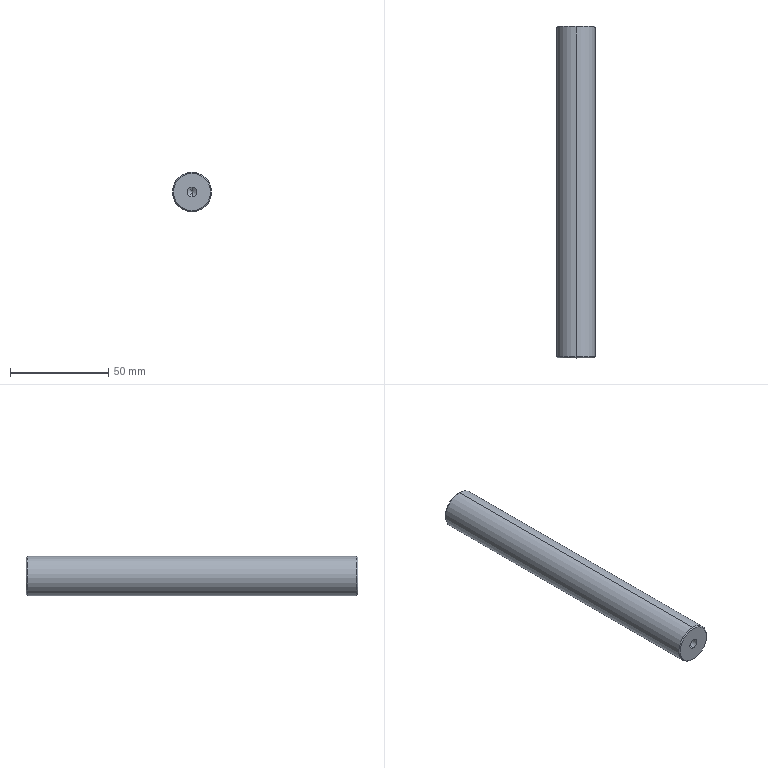Part | SolidWorks | features BaseBody 1 | 1 solid | 16 faces | box 20 x 169 x 20 mm | volume 51704 mm3 | cone 8 | cylinder 6 | plane 2 | commonest cylinder face diameters 5 x2 6.8 x2 20 x2
STEP:
#1=CARTESIAN_POINT('',(0.,15.,2.5));
#2=VERTEX_POINT('',#1);
#3=CARTESIAN_POINT('',(0.,15.,-2.5));
#4=VERTEX_POINT('',#3);
#5=CARTESIAN_POINT('',(0.,15.,0.));
#6=DIRECTION('',(0.,-1.,0.));
#7=DIRECTION('',(0.,0.,-1.));
#8=AXIS2_PLACEMENT_3D('',#5,#6,#7);
#9=CIRCLE('',#8,2.5);
#10=EDGE_CURVE('',#2,#4,#9,.T.);
#11=ORIENTED_EDGE('',*,*,#10,.F.);
#12=CARTESIAN_POINT('',(0.,0.,2.5));
#13=VERTEX_POINT('',#12);
#14=CARTESIAN_POINT('',(0.,0.,2.5));
#15=DIRECTION('',(0.,-1.,0.));
#16=VECTOR('',#15,1000.);
#17=LINE('',#14,#16);
#18=EDGE_CURVE('',#2,#13,#17,.T.);
#19=ORIENTED_EDGE('',*,*,#18,.T.);
#20=CARTESIAN_POINT('',(0.,0.,-2.5));
#21=VERTEX_POINT('',#20);
#22=CARTESIAN_POINT('',(0.,0.,0.));
#23=DIRECTION('',(0.,-1.,0.));
#24=DIRECTION('',(0.,0.,-1.));
#25=AXIS2_PLACEMENT_3D('',#22,#23,#24);
#26=CIRCLE('',#25,2.5);
#27=EDGE_CURVE('',#13,#21,#26,.T.);
#28=ORIENTED_EDGE('',*,*,#27,.T.);
#29=CARTESIAN_POINT('',(0.,0.,-2.5));
#30=DIRECTION('',(0.,-1.,0.));
#31=VECTOR('',#30,1000.);
#32=LINE('',#29,#31);
#33=EDGE_CURVE('',#4,#21,#32,.T.);
#34=ORIENTED_EDGE('',*,*,#33,.F.);
#35=EDGE_LOOP('',(#11,#19,#28,#34));
#36=FACE_OUTER_BOUND('',#35,.T.);
#37=CARTESIAN_POINT('',(0.,0.,0.));
#38=DIRECTION('',(0.,-1.,0.));
#39=DIRECTION('',(0.,0.,-1.));
#40=AXIS2_PLACEMENT_3D('',#37,#38,#39);
#41=CYLINDRICAL_SURFACE('',#40,2.5);
#42=ADVANCED_FACE('',(#36),#41,.F.);
#43=CARTESIAN_POINT('',(0.,16.502,0.));
#44=VERTEX_POINT('',#43);
#45=CARTESIAN_POINT('',(0.,15.,-2.5));
#46=DIRECTION('',(0.,-0.515,-0.8572));
#47=VECTOR('',#46,1000.);
#48=LINE('',#45,#47);
#49=EDGE_CURVE('',#44,#4,#48,.T.);
#50=ORIENTED_EDGE('',*,*,#49,.F.);
#51=CARTESIAN_POINT('',(0.,15.,2.5));
#52=DIRECTION('',(0.,-0.515,0.8572));
#53=VECTOR('',#52,1000.);
#54=LINE('',#51,#53);
#55=EDGE_CURVE('',#44,#2,#54,.T.);
#56=ORIENTED_EDGE('',*,*,#55,.T.);
#57=ORIENTED_EDGE('',*,*,#10,.T.);
#58=EDGE_LOOP('',(#50,#56,#57));
#59=FACE_OUTER_BOUND('',#58,.T.);
#60=CARTESIAN_POINT('',(0.,15.,0.));
#61=DIRECTION('',(0.,-1.,0.));
#62=DIRECTION('',(0.,0.,-1.));
#63=AXIS2_PLACEMENT_3D('',#60,#61,#62);
#64=CONICAL_SURFACE('',#63,2.5,1.03);
#65=ADVANCED_FACE('',(#59),#64,.F.);
#66=CARTESIAN_POINT('',(0.,140.25,-3.4));
#67=VERTEX_POINT('',#66);
#68=CARTESIAN_POINT('',(0.,140.25,3.4));
#69=VERTEX_POINT('',#68);
#70=CARTESIAN_POINT('',(0.,140.25,0.));
#71=DIRECTION('',(0.,1.,0.));
#72=DIRECTION('',(0.,0.,1.));
#73=AXIS2_PLACEMENT_3D('',#70,#71,#72);
#74=CIRCLE('',#73,3.4);
#75=EDGE_CURVE('',#67,#69,#74,.T.);
#76=ORIENTED_EDGE('',*,*,#75,.F.);
#77=CARTESIAN_POINT('',(0.,169.,-3.4));
#78=VERTEX_POINT('',#77);
#79=CARTESIAN_POINT('',(0.,169.,-3.4));
#80=DIRECTION('',(0.,1.,0.));
#81=VECTOR('',#80,1000.);
#82=LINE('',#79,#81);
#83=EDGE_CURVE('',#67,#78,#82,.T.);
#84=ORIENTED_EDGE('',*,*,#83,.T.);
#85=CARTESIAN_POINT('',(0.,169.,3.4));
#86=VERTEX_POINT('',#85);
#87=CARTESIAN_POINT('',(0.,169.,0.));
#88=DIRECTION('',(0.,1.,0.));
#89=DIRECTION('',(0.,0.,1.));
#90=AXIS2_PLACEMENT_3D('',#87,#88,#89);
#91=CIRCLE('',#90,3.4);
#92=EDGE_CURVE('',#78,#86,#91,.T.);
#93=ORIENTED_EDGE('',*,*,#92,.T.);
#94=CARTESIAN_POINT('',(0.,169.,3.4));
#95=DIRECTION('',(0.,1.,0.));
#96=VECTOR('',#95,1000.);
#97=LINE('',#94,#96);
#98=EDGE_CURVE('',#69,#86,#97,.T.);
#99=ORIENTED_EDGE('',*,*,#98,.F.);
#100=EDGE_LOOP('',(#76,#84,#93,#99));
#101=FACE_OUTER_BOUND('',#100,.T.);
#102=CARTESIAN_POINT('',(0.,169.,0.));
#103=DIRECTION('',(0.,1.,0.));
#104=DIRECTION('',(0.,0.,1.));
#105=AXIS2_PLACEMENT_3D('',#102,#103,#104);
#106=CYLINDRICAL_SURFACE('',#105,3.4);
#107=ADVANCED_FACE('',(#101),#106,.F.);
#108=CARTESIAN_POINT('',(0.,138.207,0.));
#109=VERTEX_POINT('',#108);
#110=CARTESIAN_POINT('',(0.,140.25,3.4));
#111=DIRECTION('',(0.,0.515,0.8572));
#112=VECTOR('',#111,1000.);
#113=LINE('',#110,#112);
#114=EDGE_CURVE('',#109,#69,#113,.T.);
#115=ORIENTED_EDGE('',*,*,#114,.F.);
#116=CARTESIAN_POINT('',(0.,140.25,-3.4));
#117=DIRECTION('',(0.,0.515,-0.8572));
#118=VECTOR('',#117,1000.);
#119=LINE('',#116,#118);
#120=EDGE_CURVE('',#109,#67,#119,.T.);
#121=ORIENTED_EDGE('',*,*,#120,.T.);
#122=ORIENTED_EDGE('',*,*,#75,.T.);
#123=EDGE_LOOP('',(#115,#121,#122));
#124=FACE_OUTER_BOUND('',#123,.T.);
#125=CARTESIAN_POINT('',(0.,140.25,0.));
#126=DIRECTION('',(0.,1.,0.));
#127=DIRECTION('',(0.,0.,1.));
#128=AXIS2_PLACEMENT_3D('',#125,#126,#127);
#129=CONICAL_SURFACE('',#128,3.4,1.03);
#130=ADVANCED_FACE('',(#124),#129,.F.);
#131=CARTESIAN_POINT('',(0.,169.,9.5));
#132=VERTEX_POINT('',#131);
#133=CARTESIAN_POINT('',(0.,169.,-9.5));
#134=VERTEX_POINT('',#133);
#135=CARTESIAN_POINT('',(0.,169.,0.));
#136=DIRECTION('',(0.,1.,0.));
#137=DIRECTION('',(0.,0.,1.));
#138=AXIS2_PLACEMENT_3D('',#135,#136,#137);
#139=CIRCLE('',#138,9.5);
#140=EDGE_CURVE('',#132,#134,#139,.T.);
#141=ORIENTED_EDGE('',*,*,#140,.F.);
#142=CARTESIAN_POINT('',(0.,168.5,10.));
#143=VERTEX_POINT('',#142);
#144=CARTESIAN_POINT('',(0.,169.,9.5));
#145=DIRECTION('',(0.,-0.7071,0.7071));
#146=VECTOR('',#145,1000.);
#147=LINE('',#144,#146);
#148=EDGE_CURVE('',#132,#143,#147,.T.);
#149=ORIENTED_EDGE('',*,*,#148,.T.);
#150=CARTESIAN_POINT('',(0.,168.5,-10.));
#151=VERTEX_POINT('',#150);
#152=CARTESIAN_POINT('',(0.,168.5,0.));
#153=DIRECTION('',(0.,-1.,0.));
#154=DIRECTION('',(0.,0.,1.));
#155=AXIS2_PLACEMENT_3D('',#152,#153,#154);
#156=CIRCLE('',#155,10.);
#157=EDGE_CURVE('',#151,#143,#156,.T.);
#158=ORIENTED_EDGE('',*,*,#157,.F.);
#159=CARTESIAN_POINT('',(0.,169.,-9.5));
#160=DIRECTION('',(0.,-0.7071,-0.7071));
#161=VECTOR('',#160,1000.);
#162=LINE('',#159,#161);
#163=EDGE_CURVE('',#134,#151,#162,.T.);
#164=ORIENTED_EDGE('',*,*,#163,.F.);
#165=EDGE_LOOP('',(#141,#149,#158,#164));
#166=FACE_OUTER_BOUND('',#165,.T.);
#167=CARTESIAN_POINT('',(0.,169.,0.));
#168=DIRECTION('',(0.,-1.,0.));
#169=DIRECTION('',(0.,0.,-1.));
#170=AXIS2_PLACEMENT_3D('',#167,#168,#169);
#171=CONICAL_SURFACE('',#170,9.5,0.7854);
#172=ADVANCED_FACE('',(#166),#171,.T.);
#173=CARTESIAN_POINT('',(0.,0.,-9.5));
#174=VERTEX_POINT('',#173);
#175=CARTESIAN_POINT('',(0.,0.,9.5));
#176=VERTEX_POINT('',#175);
#177=CARTESIAN_POINT('',(0.,0.,0.));
#178=DIRECTION('',(0.,-1.,0.));
#179=DIRECTION('',(0.,0.,1.));
#180=AXIS2_PLACEMENT_3D('',#177,#178,#179);
#181=CIRCLE('',#180,9.5);
#182=EDGE_CURVE('',#174,#176,#181,.T.);
#183=ORIENTED_EDGE('',*,*,#182,.F.);
#184=CARTESIAN_POINT('',(0.,0.5,-10.));
#185=VERTEX_POINT('',#184);
#186=CARTESIAN_POINT('',(0.,0.5,-10.));
#187=DIRECTION('',(0.,0.7071,-0.7071));
#188=VECTOR('',#187,1000.);
#189=LINE('',#186,#188);
#190=EDGE_CURVE('',#174,#185,#189,.T.);
#191=ORIENTED_EDGE('',*,*,#190,.T.);
#192=CARTESIAN_POINT('',(0.,0.5,10.));
#193=VERTEX_POINT('',#192);
#194=CARTESIAN_POINT('',(0.,0.5,0.));
#195=DIRECTION('',(0.,1.,0.));
#196=DIRECTION('',(0.,0.,1.));
#197=AXIS2_PLACEMENT_3D('',#194,#195,#196);
#198=CIRCLE('',#197,10.);
#199=EDGE_CURVE('',#193,#185,#198,.T.);
#200=ORIENTED_EDGE('',*,*,#199,.F.);
#201=CARTESIAN_POINT('',(0.,0.5,10.));
#202=DIRECTION('',(0.,0.7071,0.7071));
#203=VECTOR('',#202,1000.);
#204=LINE('',#201,#203);
#205=EDGE_CURVE('',#176,#193,#204,.T.);
#206=ORIENTED_EDGE('',*,*,#205,.F.);
#207=EDGE_LOOP('',(#183,#191,#200,#206));
#208=FACE_OUTER_BOUND('',#207,.T.);
#209=CARTESIAN_POINT('',(0.,0.5,0.));
#210=DIRECTION('',(0.,1.,0.));
#211=DIRECTION('',(0.,0.,1.));
#212=AXIS2_PLACEMENT_3D('',#209,#210,#211);
#213=CONICAL_SURFACE('',#212,10.,0.7854);
#214=ADVANCED_FACE('',(#208),#213,.T.);
#215=ORIENTED_EDGE('',*,*,#157,.T.);
#216=CARTESIAN_POINT('',(0.,169.,10.));
#217=DIRECTION('',(0.,-1.,0.));
#218=VECTOR('',#217,1000.);
#219=LINE('',#216,#218);
#220=EDGE_CURVE('',#143,#193,#219,.T.);
#221=ORIENTED_EDGE('',*,*,#220,.T.);
#222=ORIENTED_EDGE('',*,*,#199,.T.);
#223=CARTESIAN_POINT('',(0.,169.,-10.));
#224=DIRECTION('',(0.,-1.,0.));
#225=VECTOR('',#224,1000.);
#226=LINE('',#223,#225);
#227=EDGE_CURVE('',#151,#185,#226,.T.);
#228=ORIENTED_EDGE('',*,*,#227,.F.);
#229=EDGE_LOOP('',(#215,#221,#222,#228));
#230=FACE_OUTER_BOUND('',#229,.T.);
#231=CARTESIAN_POINT('',(0.,169.,0.));
#232=DIRECTION('',(0.,-1.,0.));
#233=DIRECTION('',(0.,0.,-1.));
#234=AXIS2_PLACEMENT_3D('',#231,#232,#233);
#235=CYLINDRICAL_SURFACE('',#234,10.);
#236=ADVANCED_FACE('',(#230),#235,.T.);
#237=CARTESIAN_POINT('',(0.,0.,0.));
#238=DIRECTION('',(0.,-1.,0.));
#239=DIRECTION('',(0.,0.,-1.));
#240=AXIS2_PLACEMENT_3D('',#237,#238,#239);
#241=CIRCLE('',#240,2.5);
#242=EDGE_CURVE('',#21,#13,#241,.T.);
#243=ORIENTED_EDGE('',*,*,#242,.F.);
#244=ORIENTED_EDGE('',*,*,#27,.F.);
#245=EDGE_LOOP('',(#243,#244));
#246=FACE_BOUND('',#245,.T.);
#247=CARTESIAN_POINT('',(0.,0.,0.));
#248=DIRECTION('',(0.,-1.,0.));
#249=DIRECTION('',(0.,0.,1.));
#250=AXIS2_PLACEMENT_3D('',#247,#248,#249);
#251=CIRCLE('',#250,9.5);
#252=EDGE_CURVE('',#176,#174,#251,.T.);
#253=ORIENTED_EDGE('',*,*,#252,.T.);
#254=ORIENTED_EDGE('',*,*,#182,.T.);
#255=EDGE_LOOP('',(#253,#254));
#256=FACE_OUTER_BOUND('',#255,.T.);
#257=CARTESIAN_POINT('',(0.,0.,0.));
#258=DIRECTION('',(0.,1.,0.));
#259=DIRECTION('',(1.,0.,0.));
#260=AXIS2_PLACEMENT_3D('',#257,#258,#259);
#261=PLANE('',#260);
#262=ADVANCED_FACE('',(#246,#256),#261,.F.);
#263=CARTESIAN_POINT('',(0.,169.,0.));
#264=DIRECTION('',(0.,1.,0.));
#265=DIRECTION('',(0.,0.,1.));
#266=AXIS2_PLACEMENT_3D('',#263,#264,#265);
#267=CIRCLE('',#266,3.4);
#268=EDGE_CURVE('',#86,#78,#267,.T.);
#269=ORIENTED_EDGE('',*,*,#268,.F.);
#270=ORIENTED_EDGE('',*,*,#92,.F.);
#271=EDGE_LOOP('',(#269,#270));
#272=FACE_BOUND('',#271,.T.);
#273=CARTESIAN_POINT('',(0.,169.,0.));
#274=DIRECTION('',(0.,1.,0.));
#275=DIRECTION('',(0.,0.,1.));
#276=AXIS2_PLACEMENT_3D('',#273,#274,#275);
#277=CIRCLE('',#276,9.5);
#278=EDGE_CURVE('',#134,#132,#277,.T.);
#279=ORIENTED_EDGE('',*,*,#278,.T.);
#280=ORIENTED_EDGE('',*,*,#140,.T.);
#281=EDGE_LOOP('',(#279,#280));
#282=FACE_OUTER_BOUND('',#281,.T.);
#283=CARTESIAN_POINT('',(0.,169.,0.));
#284=DIRECTION('',(0.,1.,0.));
#285=DIRECTION('',(1.,0.,0.));
#286=AXIS2_PLACEMENT_3D('',#283,#284,#285);
#287=PLANE('',#286);
#288=ADVANCED_FACE('',(#272,#282),#287,.T.);
#289=ORIENTED_EDGE('',*,*,#220,.F.);
#290=CARTESIAN_POINT('',(0.,168.5,0.));
#291=DIRECTION('',(0.,-1.,0.));
#292=DIRECTION('',(0.,0.,1.));
#293=AXIS2_PLACEMENT_3D('',#290,#291,#292);
#294=CIRCLE('',#293,10.);
#295=EDGE_CURVE('',#143,#151,#294,.T.);
#296=ORIENTED_EDGE('',*,*,#295,.T.);
#297=ORIENTED_EDGE('',*,*,#227,.T.);
#298=CARTESIAN_POINT('',(0.,0.5,0.));
#299=DIRECTION('',(0.,1.,0.));
#300=DIRECTION('',(0.,0.,1.));
#301=AXIS2_PLACEMENT_3D('',#298,#299,#300);
#302=CIRCLE('',#301,10.);
#303=EDGE_CURVE('',#185,#193,#302,.T.);
#304=ORIENTED_EDGE('',*,*,#303,.T.);
#305=EDGE_LOOP('',(#289,#296,#297,#304));
#306=FACE_OUTER_BOUND('',#305,.T.);
#307=CARTESIAN_POINT('',(0.,169.,0.));
#308=DIRECTION('',(0.,-1.,0.));
#309=DIRECTION('',(0.,0.,-1.));
#310=AXIS2_PLACEMENT_3D('',#307,#308,#309);
#311=CYLINDRICAL_SURFACE('',#310,10.);
#312=ADVANCED_FACE('',(#306),#311,.T.);
#313=ORIENTED_EDGE('',*,*,#190,.F.);
#314=ORIENTED_EDGE('',*,*,#252,.F.);
#315=ORIENTED_EDGE('',*,*,#205,.T.);
#316=ORIENTED_EDGE('',*,*,#303,.F.);
#317=EDGE_LOOP('',(#313,#314,#315,#316));
#318=FACE_OUTER_BOUND('',#317,.T.);
#319=CARTESIAN_POINT('',(0.,0.5,0.));
#320=DIRECTION('',(0.,1.,0.));
#321=DIRECTION('',(0.,0.,1.));
#322=AXIS2_PLACEMENT_3D('',#319,#320,#321);
#323=CONICAL_SURFACE('',#322,10.,0.7854);
#324=ADVANCED_FACE('',(#318),#323,.T.);
#325=ORIENTED_EDGE('',*,*,#148,.F.);
#326=ORIENTED_EDGE('',*,*,#278,.F.);
#327=ORIENTED_EDGE('',*,*,#163,.T.);
#328=ORIENTED_EDGE('',*,*,#295,.F.);
#329=EDGE_LOOP('',(#325,#326,#327,#328));
#330=FACE_OUTER_BOUND('',#329,.T.);
#331=CARTESIAN_POINT('',(0.,169.,0.));
#332=DIRECTION('',(0.,-1.,0.));
#333=DIRECTION('',(0.,0.,-1.));
#334=AXIS2_PLACEMENT_3D('',#331,#332,#333);
#335=CONICAL_SURFACE('',#334,9.5,0.7854);
#336=ADVANCED_FACE('',(#330),#335,.T.);
#337=ORIENTED_EDGE('',*,*,#120,.F.);
#338=ORIENTED_EDGE('',*,*,#114,.T.);
#339=CARTESIAN_POINT('',(0.,140.25,0.));
#340=DIRECTION('',(0.,1.,0.));
#341=DIRECTION('',(0.,0.,1.));
#342=AXIS2_PLACEMENT_3D('',#339,#340,#341);
#343=CIRCLE('',#342,3.4);
#344=EDGE_CURVE('',#69,#67,#343,.T.);
#345=ORIENTED_EDGE('',*,*,#344,.T.);
#346=EDGE_LOOP('',(#337,#338,#345));
#347=FACE_OUTER_BOUND('',#346,.T.);
#348=CARTESIAN_POINT('',(0.,140.25,0.));
#349=DIRECTION('',(0.,1.,0.));
#350=DIRECTION('',(0.,0.,1.));
#351=AXIS2_PLACEMENT_3D('',#348,#349,#350);
#352=CONICAL_SURFACE('',#351,3.4,1.03);
#353=ADVANCED_FACE('',(#347),#352,.F.);
#354=ORIENTED_EDGE('',*,*,#83,.F.);
#355=ORIENTED_EDGE('',*,*,#344,.F.);
#356=ORIENTED_EDGE('',*,*,#98,.T.);
#357=ORIENTED_EDGE('',*,*,#268,.T.);
#358=EDGE_LOOP('',(#354,#355,#356,#357));
#359=FACE_OUTER_BOUND('',#358,.T.);
#360=CARTESIAN_POINT('',(0.,169.,0.));
#361=DIRECTION('',(0.,1.,0.));
#362=DIRECTION('',(0.,0.,1.));
#363=AXIS2_PLACEMENT_3D('',#360,#361,#362);
#364=CYLINDRICAL_SURFACE('',#363,3.4);
#365=ADVANCED_FACE('',(#359),#364,.F.);
#366=ORIENTED_EDGE('',*,*,#55,.F.);
#367=ORIENTED_EDGE('',*,*,#49,.T.);
#368=CARTESIAN_POINT('',(0.,15.,0.));
#369=DIRECTION('',(0.,-1.,0.));
#370=DIRECTION('',(0.,0.,-1.));
#371=AXIS2_PLACEMENT_3D('',#368,#369,#370);
#372=CIRCLE('',#371,2.5);
#373=EDGE_CURVE('',#4,#2,#372,.T.);
#374=ORIENTED_EDGE('',*,*,#373,.T.);
#375=EDGE_LOOP('',(#366,#367,#374));
#376=FACE_OUTER_BOUND('',#375,.T.);
#377=CARTESIAN_POINT('',(0.,15.,0.));
#378=DIRECTION('',(0.,-1.,0.));
#379=DIRECTION('',(0.,0.,-1.));
#380=AXIS2_PLACEMENT_3D('',#377,#378,#379);
#381=CONICAL_SURFACE('',#380,2.5,1.03);
#382=ADVANCED_FACE('',(#376),#381,.F.);
#383=ORIENTED_EDGE('',*,*,#18,.F.);
#384=ORIENTED_EDGE('',*,*,#373,.F.);
#385=ORIENTED_EDGE('',*,*,#33,.T.);
#386=ORIENTED_EDGE('',*,*,#242,.T.);
#387=EDGE_LOOP('',(#383,#384,#385,#386));
#388=FACE_OUTER_BOUND('',#387,.T.);
#389=CARTESIAN_POINT('',(0.,0.,0.));
#390=DIRECTION('',(0.,-1.,0.));
#391=DIRECTION('',(0.,0.,-1.));
#392=AXIS2_PLACEMENT_3D('',#389,#390,#391);
#393=CYLINDRICAL_SURFACE('',#392,2.5);
#394=ADVANCED_FACE('',(#388),#393,.F.);
#395=CLOSED_SHELL('',(#42,#65,#107,#130,#172,#214,#236,#262,#288,#312,#324,#336,#353,#365,#382,#394));
#396=MANIFOLD_SOLID_BREP('',#395);
#397=CARTESIAN_POINT('',(0.,0.,0.));
#398=DIRECTION('',(0.,0.,1.));
#399=DIRECTION('',(1.,0.,0.));
#400=AXIS2_PLACEMENT_3D('',#397,#398,#399);
#401=(LENGTH_UNIT()NAMED_UNIT(*)SI_UNIT(.MILLI.,.METRE.));
#402=UNCERTAINTY_MEASURE_WITH_UNIT(LENGTH_MEASURE(0.00001),#401,'','');
#403=(NAMED_UNIT(*)PLANE_ANGLE_UNIT()SI_UNIT($,.RADIAN.));
#404=(NAMED_UNIT(*)SI_UNIT($,.STERADIAN.)SOLID_ANGLE_UNIT());
#405=(GEOMETRIC_REPRESENTATION_CONTEXT(3)GLOBAL_UNCERTAINTY_ASSIGNED_CONTEXT((#402))GLOBAL_UNIT_ASSIGNED_CONTEXT((#401,#403,#404))REPRESENTATION_CONTEXT('',''));
#406=ADVANCED_BREP_SHAPE_REPRESENTATION('',(#396,#400),#405);